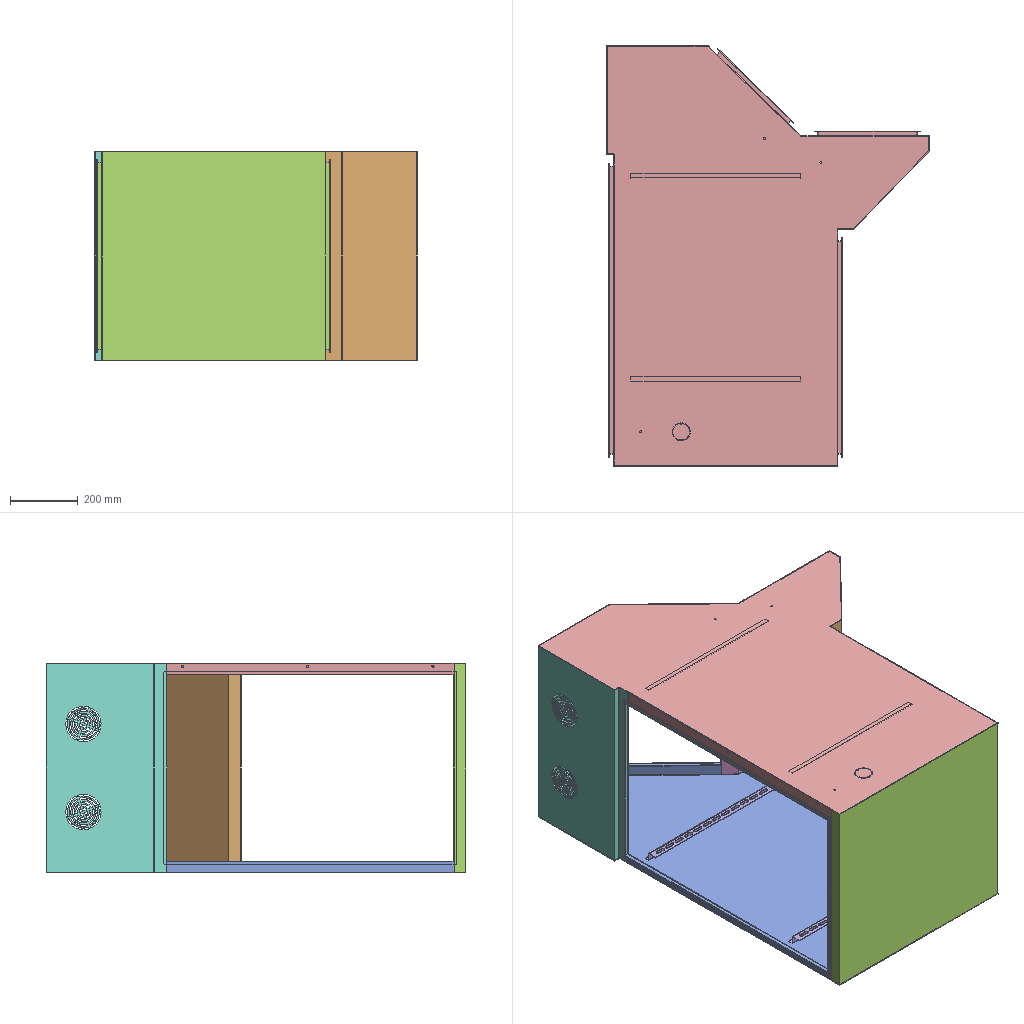Assembly | SolidWorks | 7 different items | 10 placed | box 953 x 1240 x 620 mm
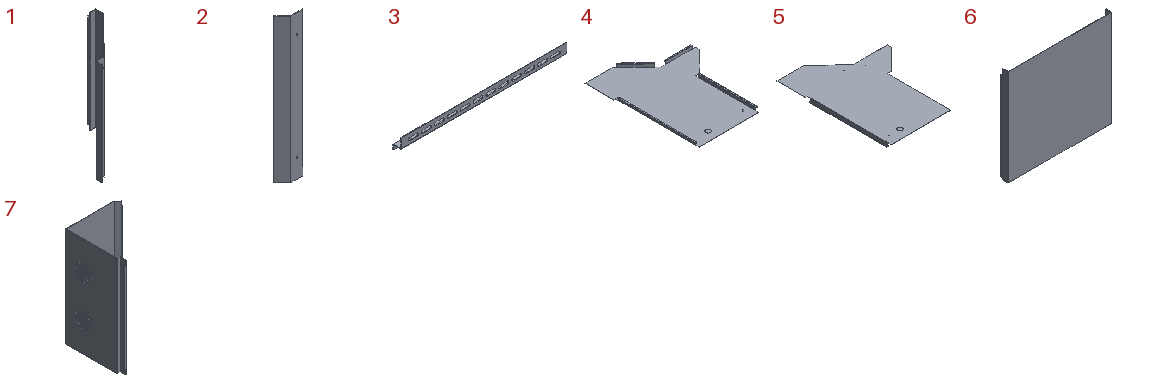Parts list (item | quantity | size | volume | features):
1 | x1 | 272.129 x 325.286 x 617 mm | 483696 mm3 | features SMBaseFlange 3, EdgeFlange 2, Fillet 1, FlatPattern 1, SheetMetal 1
2 | x1 | 88.831 x 46.399 x 617 mm | 130995 mm3 | features SMBaseFlange 3, EdgeFlange 2, Cut 1, Fillet 1, FlatPattern 1, SheetMetal 1
3 | x4 | 500 x 26 x 43 mm | 59993 mm3 | features EdgeFlange 2, FlatPattern 1, ICE 1, LPattern 1, SMBaseFlange 1, SheetMetal 1
4 | x1 | 952.629 x 1240 x 35 mm | 1386350 mm3 | features EdgeFlange 3, ICE 2, FlatPattern 1, FormToolInstance 1, SMBaseFlange 1, SheetMetal 1
5 | x1 | 952.629 x 1240 x 35 mm | 1387025 mm3 | features EdgeFlange 3, ICE 3, FlatPattern 1, FormToolInstance 1, SMBaseFlange 1, SheetMetal 1
6 | x1 | 689 x 36.5 x 617 mm | 712057 mm3 | features EdgeFlange 3, SMBaseFlange 3, Fillet 1, FlatPattern 1, SheetMetal 1
7 | x1 | 334.929 x 356.5 x 617 mm | 679567 mm3 | features SMBaseFlange 3, EdgeFlange 2, Fillet 1, FlatPattern 1, MacroFeature 1, MirrorPattern 1, SheetMetal 1
Mates (type | each side: item.copy, entity, surface, feature):
Coincident | 5.1 face plane Base-Flange1 | 3.1 face plane Edge-Flange1
DistanceDim | 3.1 face plane Base-Flange1 | 5.1 face plane Edge-Flange2
DistanceDim | 3.1 face plane Base-Flange1 | 6.1 face plane Base-Flange1
Coincident | 4.1 face plane Base-Flange1 | 3.2 face plane Edge-Flange1
Coincident | 3.1 face plane Base-Flange1 | 3.2 face plane Base-Flange1 | 2 times